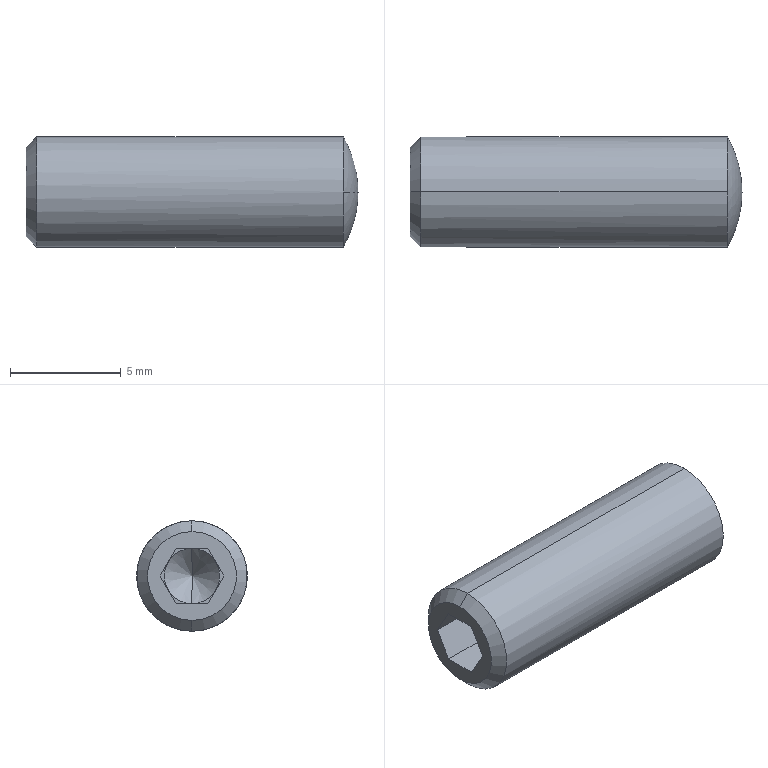Part | STEP file | Sceond1_8 | 1 solid | 21 faces | box 15 x 5 x 5 mm | volume 269.138 mm3 | plane 13 | cone 4 | spline 2 | cylinder 2 | commonest cylinder face diameters 5 x2